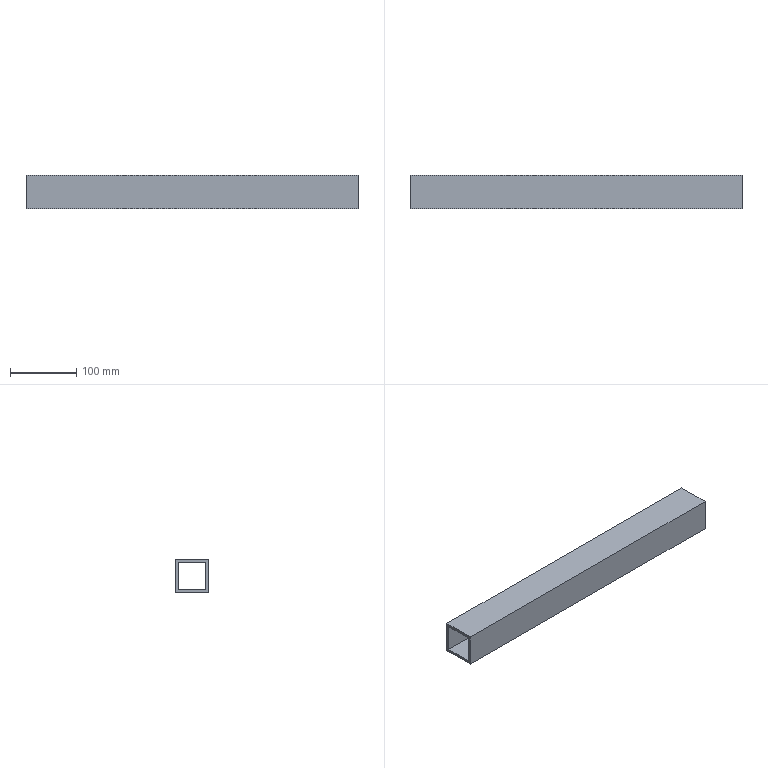Part | STEP file | PN_0084 cross stop bar | 1 solid | 10 faces | box 500 x 50 x 50 mm | volume 368000 mm3 | plane 10
STEP:
#1=CARTESIAN_POINT('',(0.,0.,0.));
#2=DIRECTION('',(0.,0.,1.));
#3=DIRECTION('',(1.,0.,0.));
#4=AXIS2_PLACEMENT_3D('',#1,#2,#3);
#5=CARTESIAN_POINT('',(500.,25.,-25.));
#6=VERTEX_POINT('',#5);
#7=CARTESIAN_POINT('',(500.,25.,25.));
#8=VERTEX_POINT('',#7);
#9=CARTESIAN_POINT('',(500.,25.,25.));
#10=DIRECTION('',(0.,0.,1.));
#11=VECTOR('',#10,1.);
#12=LINE('',#9,#11);
#13=CARTESIAN_POINT('',(500.,0.,0.));
#14=DIRECTION('',(1.,0.,0.));
#15=DIRECTION('',(0.,0.,-1.));
#16=AXIS2_PLACEMENT_3D('',#13,#14,#15);
#17=PLANE('',#16);
#18=CARTESIAN_POINT('',(-25.,25.));
#19=DIRECTION('',(-1.,0.));
#20=VECTOR('',#19,1.);
#21=LINE('',#18,#20);
#22=(GEOMETRIC_REPRESENTATION_CONTEXT(2)PARAMETRIC_REPRESENTATION_CONTEXT()REPRESENTATION_CONTEXT('',''));
#23=DEFINITIONAL_REPRESENTATION('',(#21),#22);
#24=PCURVE('',#17,#23);
#25=CARTESIAN_POINT('',(500.,25.,25.));
#26=DIRECTION('',(0.,-1.,0.));
#27=DIRECTION('',(0.,0.,-1.));
#28=AXIS2_PLACEMENT_3D('',#25,#26,#27);
#29=PLANE('',#28);
#30=CARTESIAN_POINT('',(0.,0.));
#31=DIRECTION('',(-1.,0.));
#32=VECTOR('',#31,1.);
#33=LINE('',#30,#32);
#34=(GEOMETRIC_REPRESENTATION_CONTEXT(2)PARAMETRIC_REPRESENTATION_CONTEXT()REPRESENTATION_CONTEXT('',''));
#35=DEFINITIONAL_REPRESENTATION('',(#33),#34);
#36=PCURVE('',#29,#35);
#37=SURFACE_CURVE('',#12,(#24,#36),.PCURVE_S1.);
#38=EDGE_CURVE('',#6,#8,#37,.T.);
#39=ORIENTED_EDGE('',*,*,#38,.T.);
#40=CARTESIAN_POINT('',(500.,-25.,25.));
#41=VERTEX_POINT('',#40);
#42=CARTESIAN_POINT('',(500.,-25.,25.));
#43=DIRECTION('',(0.,-1.,0.));
#44=VECTOR('',#43,1.);
#45=LINE('',#42,#44);
#46=CARTESIAN_POINT('',(-25.,-25.));
#47=DIRECTION('',(0.,-1.));
#48=VECTOR('',#47,1.);
#49=LINE('',#46,#48);
#50=(GEOMETRIC_REPRESENTATION_CONTEXT(2)PARAMETRIC_REPRESENTATION_CONTEXT()REPRESENTATION_CONTEXT('',''));
#51=DEFINITIONAL_REPRESENTATION('',(#49),#50);
#52=PCURVE('',#17,#51);
#53=CARTESIAN_POINT('',(500.,-25.,25.));
#54=DIRECTION('',(0.,0.,-1.));
#55=DIRECTION('',(0.,1.,0.));
#56=AXIS2_PLACEMENT_3D('',#53,#54,#55);
#57=PLANE('',#56);
#58=CARTESIAN_POINT('',(0.,0.));
#59=DIRECTION('',(-1.,0.));
#60=VECTOR('',#59,1.);
#61=LINE('',#58,#60);
#62=(GEOMETRIC_REPRESENTATION_CONTEXT(2)PARAMETRIC_REPRESENTATION_CONTEXT()REPRESENTATION_CONTEXT('',''));
#63=DEFINITIONAL_REPRESENTATION('',(#61),#62);
#64=PCURVE('',#57,#63);
#65=SURFACE_CURVE('',#45,(#52,#64),.PCURVE_S1.);
#66=EDGE_CURVE('',#8,#41,#65,.T.);
#67=ORIENTED_EDGE('',*,*,#66,.T.);
#68=CARTESIAN_POINT('',(500.,-25.,-25.));
#69=VERTEX_POINT('',#68);
#70=CARTESIAN_POINT('',(500.,-25.,25.));
#71=DIRECTION('',(0.,0.,-1.));
#72=VECTOR('',#71,1.);
#73=LINE('',#70,#72);
#74=CARTESIAN_POINT('',(-25.,-25.));
#75=DIRECTION('',(1.,0.));
#76=VECTOR('',#75,1.);
#77=LINE('',#74,#76);
#78=(GEOMETRIC_REPRESENTATION_CONTEXT(2)PARAMETRIC_REPRESENTATION_CONTEXT()REPRESENTATION_CONTEXT('',''));
#79=DEFINITIONAL_REPRESENTATION('',(#77),#78);
#80=PCURVE('',#17,#79);
#81=CARTESIAN_POINT('',(500.,-25.,25.));
#82=DIRECTION('',(0.,1.,0.));
#83=DIRECTION('',(0.,0.,1.));
#84=AXIS2_PLACEMENT_3D('',#81,#82,#83);
#85=PLANE('',#84);
#86=CARTESIAN_POINT('',(0.,0.));
#87=DIRECTION('',(-1.,0.));
#88=VECTOR('',#87,1.);
#89=LINE('',#86,#88);
#90=(GEOMETRIC_REPRESENTATION_CONTEXT(2)PARAMETRIC_REPRESENTATION_CONTEXT()REPRESENTATION_CONTEXT('',''));
#91=DEFINITIONAL_REPRESENTATION('',(#89),#90);
#92=PCURVE('',#85,#91);
#93=SURFACE_CURVE('',#73,(#80,#92),.PCURVE_S1.);
#94=EDGE_CURVE('',#41,#69,#93,.T.);
#95=ORIENTED_EDGE('',*,*,#94,.T.);
#96=CARTESIAN_POINT('',(500.,-25.,-25.));
#97=DIRECTION('',(0.,1.,0.));
#98=VECTOR('',#97,1.);
#99=LINE('',#96,#98);
#100=CARTESIAN_POINT('',(25.,-25.));
#101=DIRECTION('',(0.,1.));
#102=VECTOR('',#101,1.);
#103=LINE('',#100,#102);
#104=(GEOMETRIC_REPRESENTATION_CONTEXT(2)PARAMETRIC_REPRESENTATION_CONTEXT()REPRESENTATION_CONTEXT('',''));
#105=DEFINITIONAL_REPRESENTATION('',(#103),#104);
#106=PCURVE('',#17,#105);
#107=CARTESIAN_POINT('',(500.,-25.,-25.));
#108=DIRECTION('',(0.,0.,1.));
#109=DIRECTION('',(0.,-1.,0.));
#110=AXIS2_PLACEMENT_3D('',#107,#108,#109);
#111=PLANE('',#110);
#112=CARTESIAN_POINT('',(0.,0.));
#113=DIRECTION('',(-1.,0.));
#114=VECTOR('',#113,1.);
#115=LINE('',#112,#114);
#116=(GEOMETRIC_REPRESENTATION_CONTEXT(2)PARAMETRIC_REPRESENTATION_CONTEXT()REPRESENTATION_CONTEXT('',''));
#117=DEFINITIONAL_REPRESENTATION('',(#115),#116);
#118=PCURVE('',#111,#117);
#119=SURFACE_CURVE('',#99,(#106,#118),.PCURVE_S1.);
#120=EDGE_CURVE('',#69,#6,#119,.T.);
#121=ORIENTED_EDGE('',*,*,#120,.T.);
#122=EDGE_LOOP('',(#39,#67,#95,#121));
#123=FACE_BOUND('',#122,.T.);
#124=CARTESIAN_POINT('',(500.,21.,21.));
#125=VERTEX_POINT('',#124);
#126=CARTESIAN_POINT('',(500.,-21.,21.));
#127=VERTEX_POINT('',#126);
#128=CARTESIAN_POINT('',(500.,-21.,21.));
#129=DIRECTION('',(0.,-1.,0.));
#130=VECTOR('',#129,1.);
#131=LINE('',#128,#130);
#132=CARTESIAN_POINT('',(-21.,-21.));
#133=DIRECTION('',(0.,-1.));
#134=VECTOR('',#133,1.);
#135=LINE('',#132,#134);
#136=(GEOMETRIC_REPRESENTATION_CONTEXT(2)PARAMETRIC_REPRESENTATION_CONTEXT()REPRESENTATION_CONTEXT('',''));
#137=DEFINITIONAL_REPRESENTATION('',(#135),#136);
#138=PCURVE('',#17,#137);
#139=CARTESIAN_POINT('',(500.,-21.,21.));
#140=DIRECTION('',(0.,0.,-1.));
#141=DIRECTION('',(-1.,0.,0.));
#142=AXIS2_PLACEMENT_3D('',#139,#140,#141);
#143=PLANE('',#142);
#144=CARTESIAN_POINT('',(0.,0.));
#145=DIRECTION('',(0.,-1.));
#146=VECTOR('',#145,1.);
#147=LINE('',#144,#146);
#148=(GEOMETRIC_REPRESENTATION_CONTEXT(2)PARAMETRIC_REPRESENTATION_CONTEXT()REPRESENTATION_CONTEXT('',''));
#149=DEFINITIONAL_REPRESENTATION('',(#147),#148);
#150=PCURVE('',#143,#149);
#151=SURFACE_CURVE('',#131,(#138,#150),.PCURVE_S1.);
#152=EDGE_CURVE('',#125,#127,#151,.T.);
#153=ORIENTED_EDGE('',*,*,#152,.F.);
#154=CARTESIAN_POINT('',(500.,21.,-21.));
#155=VERTEX_POINT('',#154);
#156=CARTESIAN_POINT('',(500.,21.,21.));
#157=DIRECTION('',(0.,0.,1.));
#158=VECTOR('',#157,1.);
#159=LINE('',#156,#158);
#160=CARTESIAN_POINT('',(-21.,21.));
#161=DIRECTION('',(-1.,0.));
#162=VECTOR('',#161,1.);
#163=LINE('',#160,#162);
#164=(GEOMETRIC_REPRESENTATION_CONTEXT(2)PARAMETRIC_REPRESENTATION_CONTEXT()REPRESENTATION_CONTEXT('',''));
#165=DEFINITIONAL_REPRESENTATION('',(#163),#164);
#166=PCURVE('',#17,#165);
#167=CARTESIAN_POINT('',(500.,21.,21.));
#168=DIRECTION('',(0.,-1.,0.));
#169=DIRECTION('',(0.,0.,-1.));
#170=AXIS2_PLACEMENT_3D('',#167,#168,#169);
#171=PLANE('',#170);
#172=CARTESIAN_POINT('',(0.,0.));
#173=DIRECTION('',(-1.,0.));
#174=VECTOR('',#173,1.);
#175=LINE('',#172,#174);
#176=(GEOMETRIC_REPRESENTATION_CONTEXT(2)PARAMETRIC_REPRESENTATION_CONTEXT()REPRESENTATION_CONTEXT('',''));
#177=DEFINITIONAL_REPRESENTATION('',(#175),#176);
#178=PCURVE('',#171,#177);
#179=SURFACE_CURVE('',#159,(#166,#178),.PCURVE_S1.);
#180=EDGE_CURVE('',#155,#125,#179,.T.);
#181=ORIENTED_EDGE('',*,*,#180,.F.);
#182=CARTESIAN_POINT('',(500.,-21.,-21.));
#183=VERTEX_POINT('',#182);
#184=CARTESIAN_POINT('',(500.,-21.,-21.));
#185=DIRECTION('',(0.,1.,0.));
#186=VECTOR('',#185,1.);
#187=LINE('',#184,#186);
#188=CARTESIAN_POINT('',(21.,-21.));
#189=DIRECTION('',(0.,1.));
#190=VECTOR('',#189,1.);
#191=LINE('',#188,#190);
#192=(GEOMETRIC_REPRESENTATION_CONTEXT(2)PARAMETRIC_REPRESENTATION_CONTEXT()REPRESENTATION_CONTEXT('',''));
#193=DEFINITIONAL_REPRESENTATION('',(#191),#192);
#194=PCURVE('',#17,#193);
#195=CARTESIAN_POINT('',(500.,-21.,-21.));
#196=DIRECTION('',(0.,0.,1.));
#197=DIRECTION('',(1.,0.,0.));
#198=AXIS2_PLACEMENT_3D('',#195,#196,#197);
#199=PLANE('',#198);
#200=CARTESIAN_POINT('',(0.,0.));
#201=DIRECTION('',(0.,1.));
#202=VECTOR('',#201,1.);
#203=LINE('',#200,#202);
#204=(GEOMETRIC_REPRESENTATION_CONTEXT(2)PARAMETRIC_REPRESENTATION_CONTEXT()REPRESENTATION_CONTEXT('',''));
#205=DEFINITIONAL_REPRESENTATION('',(#203),#204);
#206=PCURVE('',#199,#205);
#207=SURFACE_CURVE('',#187,(#194,#206),.PCURVE_S1.);
#208=EDGE_CURVE('',#183,#155,#207,.T.);
#209=ORIENTED_EDGE('',*,*,#208,.F.);
#210=CARTESIAN_POINT('',(500.,-21.,21.));
#211=DIRECTION('',(0.,0.,-1.));
#212=VECTOR('',#211,1.);
#213=LINE('',#210,#212);
#214=CARTESIAN_POINT('',(-21.,-21.));
#215=DIRECTION('',(1.,0.));
#216=VECTOR('',#215,1.);
#217=LINE('',#214,#216);
#218=(GEOMETRIC_REPRESENTATION_CONTEXT(2)PARAMETRIC_REPRESENTATION_CONTEXT()REPRESENTATION_CONTEXT('',''));
#219=DEFINITIONAL_REPRESENTATION('',(#217),#218);
#220=PCURVE('',#17,#219);
#221=CARTESIAN_POINT('',(500.,-21.,21.));
#222=DIRECTION('',(0.,1.,0.));
#223=DIRECTION('',(0.,0.,1.));
#224=AXIS2_PLACEMENT_3D('',#221,#222,#223);
#225=PLANE('',#224);
#226=CARTESIAN_POINT('',(0.,0.));
#227=DIRECTION('',(-1.,0.));
#228=VECTOR('',#227,1.);
#229=LINE('',#226,#228);
#230=(GEOMETRIC_REPRESENTATION_CONTEXT(2)PARAMETRIC_REPRESENTATION_CONTEXT()REPRESENTATION_CONTEXT('',''));
#231=DEFINITIONAL_REPRESENTATION('',(#229),#230);
#232=PCURVE('',#225,#231);
#233=SURFACE_CURVE('',#213,(#220,#232),.PCURVE_S1.);
#234=EDGE_CURVE('',#127,#183,#233,.T.);
#235=ORIENTED_EDGE('',*,*,#234,.F.);
#236=EDGE_LOOP('',(#153,#181,#209,#235));
#237=FACE_BOUND('',#236,.T.);
#238=ADVANCED_FACE('',(#123,#237),#17,.T.);
#239=CARTESIAN_POINT('',(0.,25.,-25.));
#240=VERTEX_POINT('',#239);
#241=CARTESIAN_POINT('',(0.,25.,25.));
#242=VERTEX_POINT('',#241);
#243=CARTESIAN_POINT('',(0.,25.,25.));
#244=DIRECTION('',(0.,0.,1.));
#245=VECTOR('',#244,1.);
#246=LINE('',#243,#245);
#247=CARTESIAN_POINT('',(0.,0.,0.));
#248=DIRECTION('',(1.,0.,0.));
#249=DIRECTION('',(0.,0.,-1.));
#250=AXIS2_PLACEMENT_3D('',#247,#248,#249);
#251=PLANE('',#250);
#252=CARTESIAN_POINT('',(-25.,25.));
#253=DIRECTION('',(-1.,0.));
#254=VECTOR('',#253,1.);
#255=LINE('',#252,#254);
#256=(GEOMETRIC_REPRESENTATION_CONTEXT(2)PARAMETRIC_REPRESENTATION_CONTEXT()REPRESENTATION_CONTEXT('',''));
#257=DEFINITIONAL_REPRESENTATION('',(#255),#256);
#258=PCURVE('',#251,#257);
#259=CARTESIAN_POINT('',(0.,-500.));
#260=DIRECTION('',(-1.,0.));
#261=VECTOR('',#260,1.);
#262=LINE('',#259,#261);
#263=(GEOMETRIC_REPRESENTATION_CONTEXT(2)PARAMETRIC_REPRESENTATION_CONTEXT()REPRESENTATION_CONTEXT('',''));
#264=DEFINITIONAL_REPRESENTATION('',(#262),#263);
#265=PCURVE('',#29,#264);
#266=SURFACE_CURVE('',#246,(#258,#265),.PCURVE_S1.);
#267=EDGE_CURVE('',#240,#242,#266,.T.);
#268=ORIENTED_EDGE('',*,*,#267,.F.);
#269=CARTESIAN_POINT('',(0.,-25.,-25.));
#270=VERTEX_POINT('',#269);
#271=CARTESIAN_POINT('',(0.,-25.,-25.));
#272=DIRECTION('',(0.,1.,0.));
#273=VECTOR('',#272,1.);
#274=LINE('',#271,#273);
#275=CARTESIAN_POINT('',(25.,-25.));
#276=DIRECTION('',(0.,1.));
#277=VECTOR('',#276,1.);
#278=LINE('',#275,#277);
#279=(GEOMETRIC_REPRESENTATION_CONTEXT(2)PARAMETRIC_REPRESENTATION_CONTEXT()REPRESENTATION_CONTEXT('',''));
#280=DEFINITIONAL_REPRESENTATION('',(#278),#279);
#281=PCURVE('',#251,#280);
#282=CARTESIAN_POINT('',(0.,-500.));
#283=DIRECTION('',(-1.,0.));
#284=VECTOR('',#283,1.);
#285=LINE('',#282,#284);
#286=(GEOMETRIC_REPRESENTATION_CONTEXT(2)PARAMETRIC_REPRESENTATION_CONTEXT()REPRESENTATION_CONTEXT('',''));
#287=DEFINITIONAL_REPRESENTATION('',(#285),#286);
#288=PCURVE('',#111,#287);
#289=SURFACE_CURVE('',#274,(#281,#288),.PCURVE_S1.);
#290=EDGE_CURVE('',#270,#240,#289,.T.);
#291=ORIENTED_EDGE('',*,*,#290,.F.);
#292=CARTESIAN_POINT('',(0.,-25.,25.));
#293=VERTEX_POINT('',#292);
#294=CARTESIAN_POINT('',(0.,-25.,25.));
#295=DIRECTION('',(0.,0.,-1.));
#296=VECTOR('',#295,1.);
#297=LINE('',#294,#296);
#298=CARTESIAN_POINT('',(-25.,-25.));
#299=DIRECTION('',(1.,0.));
#300=VECTOR('',#299,1.);
#301=LINE('',#298,#300);
#302=(GEOMETRIC_REPRESENTATION_CONTEXT(2)PARAMETRIC_REPRESENTATION_CONTEXT()REPRESENTATION_CONTEXT('',''));
#303=DEFINITIONAL_REPRESENTATION('',(#301),#302);
#304=PCURVE('',#251,#303);
#305=CARTESIAN_POINT('',(0.,-500.));
#306=DIRECTION('',(-1.,0.));
#307=VECTOR('',#306,1.);
#308=LINE('',#305,#307);
#309=(GEOMETRIC_REPRESENTATION_CONTEXT(2)PARAMETRIC_REPRESENTATION_CONTEXT()REPRESENTATION_CONTEXT('',''));
#310=DEFINITIONAL_REPRESENTATION('',(#308),#309);
#311=PCURVE('',#85,#310);
#312=SURFACE_CURVE('',#297,(#304,#311),.PCURVE_S1.);
#313=EDGE_CURVE('',#293,#270,#312,.T.);
#314=ORIENTED_EDGE('',*,*,#313,.F.);
#315=CARTESIAN_POINT('',(0.,-25.,25.));
#316=DIRECTION('',(0.,-1.,0.));
#317=VECTOR('',#316,1.);
#318=LINE('',#315,#317);
#319=CARTESIAN_POINT('',(-25.,-25.));
#320=DIRECTION('',(0.,-1.));
#321=VECTOR('',#320,1.);
#322=LINE('',#319,#321);
#323=(GEOMETRIC_REPRESENTATION_CONTEXT(2)PARAMETRIC_REPRESENTATION_CONTEXT()REPRESENTATION_CONTEXT('',''));
#324=DEFINITIONAL_REPRESENTATION('',(#322),#323);
#325=PCURVE('',#251,#324);
#326=CARTESIAN_POINT('',(0.,-500.));
#327=DIRECTION('',(-1.,0.));
#328=VECTOR('',#327,1.);
#329=LINE('',#326,#328);
#330=(GEOMETRIC_REPRESENTATION_CONTEXT(2)PARAMETRIC_REPRESENTATION_CONTEXT()REPRESENTATION_CONTEXT('',''));
#331=DEFINITIONAL_REPRESENTATION('',(#329),#330);
#332=PCURVE('',#57,#331);
#333=SURFACE_CURVE('',#318,(#325,#332),.PCURVE_S1.);
#334=EDGE_CURVE('',#242,#293,#333,.T.);
#335=ORIENTED_EDGE('',*,*,#334,.F.);
#336=EDGE_LOOP('',(#268,#291,#314,#335));
#337=FACE_BOUND('',#336,.T.);
#338=CARTESIAN_POINT('',(0.,21.,-21.));
#339=VERTEX_POINT('',#338);
#340=CARTESIAN_POINT('',(0.,21.,21.));
#341=VERTEX_POINT('',#340);
#342=CARTESIAN_POINT('',(0.,21.,21.));
#343=DIRECTION('',(0.,0.,1.));
#344=VECTOR('',#343,1.);
#345=LINE('',#342,#344);
#346=CARTESIAN_POINT('',(-21.,21.));
#347=DIRECTION('',(-1.,0.));
#348=VECTOR('',#347,1.);
#349=LINE('',#346,#348);
#350=(GEOMETRIC_REPRESENTATION_CONTEXT(2)PARAMETRIC_REPRESENTATION_CONTEXT()REPRESENTATION_CONTEXT('',''));
#351=DEFINITIONAL_REPRESENTATION('',(#349),#350);
#352=PCURVE('',#251,#351);
#353=CARTESIAN_POINT('',(0.,-500.));
#354=DIRECTION('',(-1.,0.));
#355=VECTOR('',#354,1.);
#356=LINE('',#353,#355);
#357=(GEOMETRIC_REPRESENTATION_CONTEXT(2)PARAMETRIC_REPRESENTATION_CONTEXT()REPRESENTATION_CONTEXT('',''));
#358=DEFINITIONAL_REPRESENTATION('',(#356),#357);
#359=PCURVE('',#171,#358);
#360=SURFACE_CURVE('',#345,(#352,#359),.PCURVE_S1.);
#361=EDGE_CURVE('',#339,#341,#360,.T.);
#362=ORIENTED_EDGE('',*,*,#361,.T.);
#363=CARTESIAN_POINT('',(0.,-21.,21.));
#364=VERTEX_POINT('',#363);
#365=CARTESIAN_POINT('',(0.,-21.,21.));
#366=DIRECTION('',(0.,-1.,0.));
#367=VECTOR('',#366,1.);
#368=LINE('',#365,#367);
#369=CARTESIAN_POINT('',(-21.,-21.));
#370=DIRECTION('',(0.,-1.));
#371=VECTOR('',#370,1.);
#372=LINE('',#369,#371);
#373=(GEOMETRIC_REPRESENTATION_CONTEXT(2)PARAMETRIC_REPRESENTATION_CONTEXT()REPRESENTATION_CONTEXT('',''));
#374=DEFINITIONAL_REPRESENTATION('',(#372),#373);
#375=PCURVE('',#251,#374);
#376=CARTESIAN_POINT('',(500.,0.));
#377=DIRECTION('',(0.,-1.));
#378=VECTOR('',#377,1.);
#379=LINE('',#376,#378);
#380=(GEOMETRIC_REPRESENTATION_CONTEXT(2)PARAMETRIC_REPRESENTATION_CONTEXT()REPRESENTATION_CONTEXT('',''));
#381=DEFINITIONAL_REPRESENTATION('',(#379),#380);
#382=PCURVE('',#143,#381);
#383=SURFACE_CURVE('',#368,(#375,#382),.PCURVE_S1.);
#384=EDGE_CURVE('',#341,#364,#383,.T.);
#385=ORIENTED_EDGE('',*,*,#384,.T.);
#386=CARTESIAN_POINT('',(0.,-21.,-21.));
#387=VERTEX_POINT('',#386);
#388=CARTESIAN_POINT('',(0.,-21.,21.));
#389=DIRECTION('',(0.,0.,-1.));
#390=VECTOR('',#389,1.);
#391=LINE('',#388,#390);
#392=CARTESIAN_POINT('',(-21.,-21.));
#393=DIRECTION('',(1.,0.));
#394=VECTOR('',#393,1.);
#395=LINE('',#392,#394);
#396=(GEOMETRIC_REPRESENTATION_CONTEXT(2)PARAMETRIC_REPRESENTATION_CONTEXT()REPRESENTATION_CONTEXT('',''));
#397=DEFINITIONAL_REPRESENTATION('',(#395),#396);
#398=PCURVE('',#251,#397);
#399=CARTESIAN_POINT('',(0.,-500.));
#400=DIRECTION('',(-1.,0.));
#401=VECTOR('',#400,1.);
#402=LINE('',#399,#401);
#403=(GEOMETRIC_REPRESENTATION_CONTEXT(2)PARAMETRIC_REPRESENTATION_CONTEXT()REPRESENTATION_CONTEXT('',''));
#404=DEFINITIONAL_REPRESENTATION('',(#402),#403);
#405=PCURVE('',#225,#404);
#406=SURFACE_CURVE('',#391,(#398,#405),.PCURVE_S1.);
#407=EDGE_CURVE('',#364,#387,#406,.T.);
#408=ORIENTED_EDGE('',*,*,#407,.T.);
#409=CARTESIAN_POINT('',(0.,-21.,-21.));
#410=DIRECTION('',(0.,1.,0.));
#411=VECTOR('',#410,1.);
#412=LINE('',#409,#411);
#413=CARTESIAN_POINT('',(21.,-21.));
#414=DIRECTION('',(0.,1.));
#415=VECTOR('',#414,1.);
#416=LINE('',#413,#415);
#417=(GEOMETRIC_REPRESENTATION_CONTEXT(2)PARAMETRIC_REPRESENTATION_CONTEXT()REPRESENTATION_CONTEXT('',''));
#418=DEFINITIONAL_REPRESENTATION('',(#416),#417);
#419=PCURVE('',#251,#418);
#420=CARTESIAN_POINT('',(-500.,0.));
#421=DIRECTION('',(0.,1.));
#422=VECTOR('',#421,1.);
#423=LINE('',#420,#422);
#424=(GEOMETRIC_REPRESENTATION_CONTEXT(2)PARAMETRIC_REPRESENTATION_CONTEXT()REPRESENTATION_CONTEXT('',''));
#425=DEFINITIONAL_REPRESENTATION('',(#423),#424);
#426=PCURVE('',#199,#425);
#427=SURFACE_CURVE('',#412,(#419,#426),.PCURVE_S1.);
#428=EDGE_CURVE('',#387,#339,#427,.T.);
#429=ORIENTED_EDGE('',*,*,#428,.T.);
#430=EDGE_LOOP('',(#362,#385,#408,#429));
#431=FACE_BOUND('',#430,.T.);
#432=ADVANCED_FACE('',(#337,#431),#251,.F.);
#433=ORIENTED_EDGE('',*,*,#267,.T.);
#434=CARTESIAN_POINT('',(500.,25.,25.));
#435=DIRECTION('',(-1.,0.,0.));
#436=VECTOR('',#435,1.);
#437=LINE('',#434,#436);
#438=CARTESIAN_POINT('',(0.,0.));
#439=DIRECTION('',(0.,-1.));
#440=VECTOR('',#439,1.);
#441=LINE('',#438,#440);
#442=(GEOMETRIC_REPRESENTATION_CONTEXT(2)PARAMETRIC_REPRESENTATION_CONTEXT()REPRESENTATION_CONTEXT('',''));
#443=DEFINITIONAL_REPRESENTATION('',(#441),#442);
#444=PCURVE('',#29,#443);
#445=CARTESIAN_POINT('',(50.,0.));
#446=DIRECTION('',(0.,-1.));
#447=VECTOR('',#446,1.);
#448=LINE('',#445,#447);
#449=(GEOMETRIC_REPRESENTATION_CONTEXT(2)PARAMETRIC_REPRESENTATION_CONTEXT()REPRESENTATION_CONTEXT('',''));
#450=DEFINITIONAL_REPRESENTATION('',(#448),#449);
#451=PCURVE('',#57,#450);
#452=SURFACE_CURVE('',#437,(#444,#451),.PCURVE_S1.);
#453=EDGE_CURVE('',#8,#242,#452,.T.);
#454=ORIENTED_EDGE('',*,*,#453,.F.);
#455=ORIENTED_EDGE('',*,*,#38,.F.);
#456=CARTESIAN_POINT('',(500.,25.,-25.));
#457=DIRECTION('',(-1.,0.,0.));
#458=VECTOR('',#457,1.);
#459=LINE('',#456,#458);
#460=CARTESIAN_POINT('',(50.,0.));
#461=DIRECTION('',(0.,-1.));
#462=VECTOR('',#461,1.);
#463=LINE('',#460,#462);
#464=(GEOMETRIC_REPRESENTATION_CONTEXT(2)PARAMETRIC_REPRESENTATION_CONTEXT()REPRESENTATION_CONTEXT('',''));
#465=DEFINITIONAL_REPRESENTATION('',(#463),#464);
#466=PCURVE('',#29,#465);
#467=CARTESIAN_POINT('',(-50.,0.));
#468=DIRECTION('',(0.,-1.));
#469=VECTOR('',#468,1.);
#470=LINE('',#467,#469);
#471=(GEOMETRIC_REPRESENTATION_CONTEXT(2)PARAMETRIC_REPRESENTATION_CONTEXT()REPRESENTATION_CONTEXT('',''));
#472=DEFINITIONAL_REPRESENTATION('',(#470),#471);
#473=PCURVE('',#111,#472);
#474=SURFACE_CURVE('',#459,(#466,#473),.PCURVE_S1.);
#475=EDGE_CURVE('',#6,#240,#474,.T.);
#476=ORIENTED_EDGE('',*,*,#475,.T.);
#477=EDGE_LOOP('',(#433,#454,#455,#476));
#478=FACE_BOUND('',#477,.T.);
#479=ADVANCED_FACE('',(#478),#29,.F.);
#480=ORIENTED_EDGE('',*,*,#334,.T.);
#481=CARTESIAN_POINT('',(500.,-25.,25.));
#482=DIRECTION('',(-1.,0.,0.));
#483=VECTOR('',#482,1.);
#484=LINE('',#481,#483);
#485=CARTESIAN_POINT('',(0.,0.));
#486=DIRECTION('',(0.,-1.));
#487=VECTOR('',#486,1.);
#488=LINE('',#485,#487);
#489=(GEOMETRIC_REPRESENTATION_CONTEXT(2)PARAMETRIC_REPRESENTATION_CONTEXT()REPRESENTATION_CONTEXT('',''));
#490=DEFINITIONAL_REPRESENTATION('',(#488),#489);
#491=PCURVE('',#57,#490);
#492=CARTESIAN_POINT('',(0.,0.));
#493=DIRECTION('',(0.,-1.));
#494=VECTOR('',#493,1.);
#495=LINE('',#492,#494);
#496=(GEOMETRIC_REPRESENTATION_CONTEXT(2)PARAMETRIC_REPRESENTATION_CONTEXT()REPRESENTATION_CONTEXT('',''));
#497=DEFINITIONAL_REPRESENTATION('',(#495),#496);
#498=PCURVE('',#85,#497);
#499=SURFACE_CURVE('',#484,(#491,#498),.PCURVE_S1.);
#500=EDGE_CURVE('',#41,#293,#499,.T.);
#501=ORIENTED_EDGE('',*,*,#500,.F.);
#502=ORIENTED_EDGE('',*,*,#66,.F.);
#503=ORIENTED_EDGE('',*,*,#453,.T.);
#504=EDGE_LOOP('',(#480,#501,#502,#503));
#505=FACE_BOUND('',#504,.T.);
#506=ADVANCED_FACE('',(#505),#57,.F.);
#507=ORIENTED_EDGE('',*,*,#313,.T.);
#508=CARTESIAN_POINT('',(500.,-25.,-25.));
#509=DIRECTION('',(-1.,0.,0.));
#510=VECTOR('',#509,1.);
#511=LINE('',#508,#510);
#512=CARTESIAN_POINT('',(-50.,0.));
#513=DIRECTION('',(0.,-1.));
#514=VECTOR('',#513,1.);
#515=LINE('',#512,#514);
#516=(GEOMETRIC_REPRESENTATION_CONTEXT(2)PARAMETRIC_REPRESENTATION_CONTEXT()REPRESENTATION_CONTEXT('',''));
#517=DEFINITIONAL_REPRESENTATION('',(#515),#516);
#518=PCURVE('',#85,#517);
#519=CARTESIAN_POINT('',(0.,0.));
#520=DIRECTION('',(0.,-1.));
#521=VECTOR('',#520,1.);
#522=LINE('',#519,#521);
#523=(GEOMETRIC_REPRESENTATION_CONTEXT(2)PARAMETRIC_REPRESENTATION_CONTEXT()REPRESENTATION_CONTEXT('',''));
#524=DEFINITIONAL_REPRESENTATION('',(#522),#523);
#525=PCURVE('',#111,#524);
#526=SURFACE_CURVE('',#511,(#518,#525),.PCURVE_S1.);
#527=EDGE_CURVE('',#69,#270,#526,.T.);
#528=ORIENTED_EDGE('',*,*,#527,.F.);
#529=ORIENTED_EDGE('',*,*,#94,.F.);
#530=ORIENTED_EDGE('',*,*,#500,.T.);
#531=EDGE_LOOP('',(#507,#528,#529,#530));
#532=FACE_BOUND('',#531,.T.);
#533=ADVANCED_FACE('',(#532),#85,.F.);
#534=ORIENTED_EDGE('',*,*,#290,.T.);
#535=ORIENTED_EDGE('',*,*,#475,.F.);
#536=ORIENTED_EDGE('',*,*,#120,.F.);
#537=ORIENTED_EDGE('',*,*,#527,.T.);
#538=EDGE_LOOP('',(#534,#535,#536,#537));
#539=FACE_BOUND('',#538,.T.);
#540=ADVANCED_FACE('',(#539),#111,.F.);
#541=ORIENTED_EDGE('',*,*,#361,.F.);
#542=CARTESIAN_POINT('',(500.,21.,-21.));
#543=DIRECTION('',(-1.,0.,0.));
#544=VECTOR('',#543,1.);
#545=LINE('',#542,#544);
#546=CARTESIAN_POINT('',(42.,0.));
#547=DIRECTION('',(0.,-1.));
#548=VECTOR('',#547,1.);
#549=LINE('',#546,#548);
#550=(GEOMETRIC_REPRESENTATION_CONTEXT(2)PARAMETRIC_REPRESENTATION_CONTEXT()REPRESENTATION_CONTEXT('',''));
#551=DEFINITIONAL_REPRESENTATION('',(#549),#550);
#552=PCURVE('',#171,#551);
#553=CARTESIAN_POINT('',(0.,42.));
#554=DIRECTION('',(-1.,0.));
#555=VECTOR('',#554,1.);
#556=LINE('',#553,#555);
#557=(GEOMETRIC_REPRESENTATION_CONTEXT(2)PARAMETRIC_REPRESENTATION_CONTEXT()REPRESENTATION_CONTEXT('',''));
#558=DEFINITIONAL_REPRESENTATION('',(#556),#557);
#559=PCURVE('',#199,#558);
#560=SURFACE_CURVE('',#545,(#552,#559),.PCURVE_S1.);
#561=EDGE_CURVE('',#155,#339,#560,.T.);
#562=ORIENTED_EDGE('',*,*,#561,.F.);
#563=ORIENTED_EDGE('',*,*,#180,.T.);
#564=CARTESIAN_POINT('',(500.,21.,21.));
#565=DIRECTION('',(-1.,0.,0.));
#566=VECTOR('',#565,1.);
#567=LINE('',#564,#566);
#568=CARTESIAN_POINT('',(0.,0.));
#569=DIRECTION('',(0.,-1.));
#570=VECTOR('',#569,1.);
#571=LINE('',#568,#570);
#572=(GEOMETRIC_REPRESENTATION_CONTEXT(2)PARAMETRIC_REPRESENTATION_CONTEXT()REPRESENTATION_CONTEXT('',''));
#573=DEFINITIONAL_REPRESENTATION('',(#571),#572);
#574=PCURVE('',#171,#573);
#575=CARTESIAN_POINT('',(0.,42.));
#576=DIRECTION('',(1.,0.));
#577=VECTOR('',#576,1.);
#578=LINE('',#575,#577);
#579=(GEOMETRIC_REPRESENTATION_CONTEXT(2)PARAMETRIC_REPRESENTATION_CONTEXT()REPRESENTATION_CONTEXT('',''));
#580=DEFINITIONAL_REPRESENTATION('',(#578),#579);
#581=PCURVE('',#143,#580);
#582=SURFACE_CURVE('',#567,(#574,#581),.PCURVE_S1.);
#583=EDGE_CURVE('',#125,#341,#582,.T.);
#584=ORIENTED_EDGE('',*,*,#583,.T.);
#585=EDGE_LOOP('',(#541,#562,#563,#584));
#586=FACE_BOUND('',#585,.T.);
#587=ADVANCED_FACE('',(#586),#171,.T.);
#588=ORIENTED_EDGE('',*,*,#384,.F.);
#589=ORIENTED_EDGE('',*,*,#583,.F.);
#590=ORIENTED_EDGE('',*,*,#152,.T.);
#591=CARTESIAN_POINT('',(500.,-21.,21.));
#592=DIRECTION('',(-1.,0.,0.));
#593=VECTOR('',#592,1.);
#594=LINE('',#591,#593);
#595=CARTESIAN_POINT('',(0.,0.));
#596=DIRECTION('',(1.,0.));
#597=VECTOR('',#596,1.);
#598=LINE('',#595,#597);
#599=(GEOMETRIC_REPRESENTATION_CONTEXT(2)PARAMETRIC_REPRESENTATION_CONTEXT()REPRESENTATION_CONTEXT('',''));
#600=DEFINITIONAL_REPRESENTATION('',(#598),#599);
#601=PCURVE('',#143,#600);
#602=CARTESIAN_POINT('',(0.,0.));
#603=DIRECTION('',(0.,-1.));
#604=VECTOR('',#603,1.);
#605=LINE('',#602,#604);
#606=(GEOMETRIC_REPRESENTATION_CONTEXT(2)PARAMETRIC_REPRESENTATION_CONTEXT()REPRESENTATION_CONTEXT('',''));
#607=DEFINITIONAL_REPRESENTATION('',(#605),#606);
#608=PCURVE('',#225,#607);
#609=SURFACE_CURVE('',#594,(#601,#608),.PCURVE_S1.);
#610=EDGE_CURVE('',#127,#364,#609,.T.);
#611=ORIENTED_EDGE('',*,*,#610,.T.);
#612=EDGE_LOOP('',(#588,#589,#590,#611));
#613=FACE_BOUND('',#612,.T.);
#614=ADVANCED_FACE('',(#613),#143,.T.);
#615=ORIENTED_EDGE('',*,*,#407,.F.);
#616=ORIENTED_EDGE('',*,*,#610,.F.);
#617=ORIENTED_EDGE('',*,*,#234,.T.);
#618=CARTESIAN_POINT('',(500.,-21.,-21.));
#619=DIRECTION('',(-1.,0.,0.));
#620=VECTOR('',#619,1.);
#621=LINE('',#618,#620);
#622=CARTESIAN_POINT('',(-42.,0.));
#623=DIRECTION('',(0.,-1.));
#624=VECTOR('',#623,1.);
#625=LINE('',#622,#624);
#626=(GEOMETRIC_REPRESENTATION_CONTEXT(2)PARAMETRIC_REPRESENTATION_CONTEXT()REPRESENTATION_CONTEXT('',''));
#627=DEFINITIONAL_REPRESENTATION('',(#625),#626);
#628=PCURVE('',#225,#627);
#629=CARTESIAN_POINT('',(0.,0.));
#630=DIRECTION('',(-1.,0.));
#631=VECTOR('',#630,1.);
#632=LINE('',#629,#631);
#633=(GEOMETRIC_REPRESENTATION_CONTEXT(2)PARAMETRIC_REPRESENTATION_CONTEXT()REPRESENTATION_CONTEXT('',''));
#634=DEFINITIONAL_REPRESENTATION('',(#632),#633);
#635=PCURVE('',#199,#634);
#636=SURFACE_CURVE('',#621,(#628,#635),.PCURVE_S1.);
#637=EDGE_CURVE('',#183,#387,#636,.T.);
#638=ORIENTED_EDGE('',*,*,#637,.T.);
#639=EDGE_LOOP('',(#615,#616,#617,#638));
#640=FACE_BOUND('',#639,.T.);
#641=ADVANCED_FACE('',(#640),#225,.T.);
#642=ORIENTED_EDGE('',*,*,#428,.F.);
#643=ORIENTED_EDGE('',*,*,#637,.F.);
#644=ORIENTED_EDGE('',*,*,#208,.T.);
#645=ORIENTED_EDGE('',*,*,#561,.T.);
#646=EDGE_LOOP('',(#642,#643,#644,#645));
#647=FACE_BOUND('',#646,.T.);
#648=ADVANCED_FACE('',(#647),#199,.T.);
#649=CLOSED_SHELL('',(#238,#432,#479,#506,#533,#540,#587,#614,#641,#648));
#650=MANIFOLD_SOLID_BREP('',#649);
#651=(LENGTH_UNIT()NAMED_UNIT(*)SI_UNIT(.MILLI.,.METRE.));
#652=UNCERTAINTY_MEASURE_WITH_UNIT(LENGTH_MEASURE(0.0000001),#651,'','');
#653=(NAMED_UNIT(*)PLANE_ANGLE_UNIT()SI_UNIT($,.RADIAN.));
#654=(NAMED_UNIT(*)SI_UNIT($,.STERADIAN.)SOLID_ANGLE_UNIT());
#655=(GEOMETRIC_REPRESENTATION_CONTEXT(3)GLOBAL_UNCERTAINTY_ASSIGNED_CONTEXT((#652))GLOBAL_UNIT_ASSIGNED_CONTEXT((#651,#653,#654))REPRESENTATION_CONTEXT('',''));
#656=ADVANCED_BREP_SHAPE_REPRESENTATION('',(#4,#650),#655);